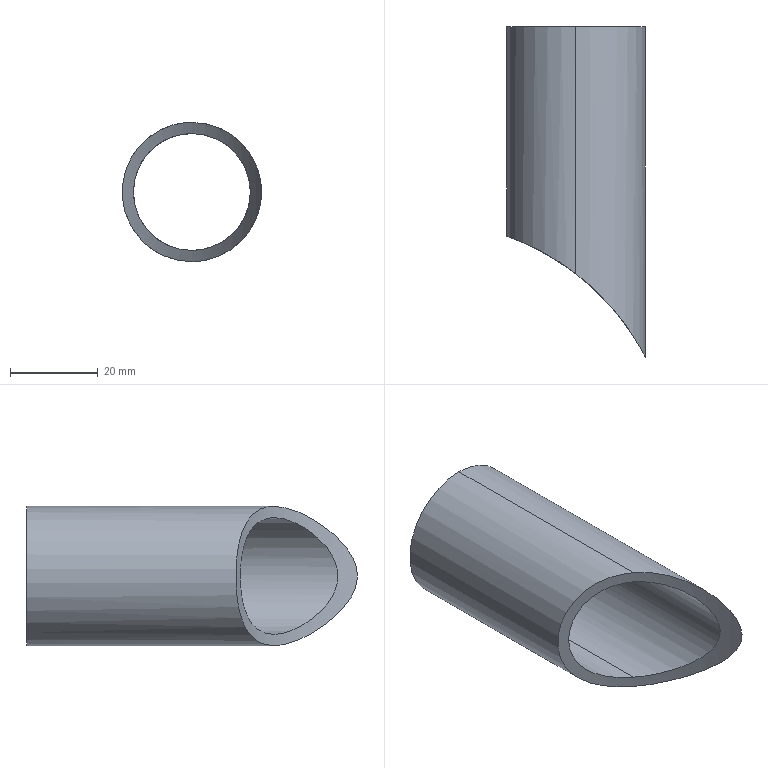Part | SolidWorks | features Extrusion 1 | 1 solid | 6 faces | box 31.75 x 75.418 x 31.75 mm | volume 13690 mm3 | cylinder 5 | plane 1 | commonest cylinder face diameters 26.645 x2 31.75 x2 114.3 x1
STEP:
#1=CARTESIAN_POINT('',(34.925,45.237,-203.822));
#2=VERTEX_POINT('',#1);
#3=CARTESIAN_POINT('',(34.925,45.237,-177.178));
#4=VERTEX_POINT('',#3);
#5=CARTESIAN_POINT('',(34.925,45.237,-203.822));
#6=CARTESIAN_POINT('',(34.177,45.814,-203.822));
#7=CARTESIAN_POINT('',(33.42,46.369,-203.76));
#8=CARTESIAN_POINT('',(32.272,47.169,-203.561));
#9=CARTESIAN_POINT('',(31.887,47.429,-203.477));
#10=CARTESIAN_POINT('',(31.114,47.94,-203.272));
#11=CARTESIAN_POINT('',(30.725,48.19,-203.15));
#12=CARTESIAN_POINT('',(29.574,48.911,-202.728));
#13=CARTESIAN_POINT('',(28.824,49.356,-202.373));
#14=CARTESIAN_POINT('',(27.729,49.974,-201.72));
#15=CARTESIAN_POINT('',(27.37,50.171,-201.482));
#16=CARTESIAN_POINT('',(26.664,50.55,-200.961));
#17=CARTESIAN_POINT('',(26.324,50.728,-200.683));
#18=CARTESIAN_POINT('',(25.343,51.229,-199.797));
#19=CARTESIAN_POINT('',(24.741,51.52,-199.138));
#20=CARTESIAN_POINT('',(23.93,51.9,-198.036));
#21=CARTESIAN_POINT('',(23.673,52.017,-197.648));
#22=CARTESIAN_POINT('',(23.204,52.228,-196.849));
#23=CARTESIAN_POINT('',(22.99,52.322,-196.438));
#24=CARTESIAN_POINT('',(22.607,52.489,-195.595));
#25=CARTESIAN_POINT('',(22.436,52.562,-195.162));
#26=CARTESIAN_POINT('',(22.14,52.688,-194.273));
#27=CARTESIAN_POINT('',(22.013,52.741,-193.815));
#28=CARTESIAN_POINT('',(21.708,52.867,-192.423));
#29=CARTESIAN_POINT('',(21.606,52.909,-191.486));
#30=CARTESIAN_POINT('',(21.601,52.91,-190.067));
#31=CARTESIAN_POINT('',(21.625,52.901,-189.589));
#32=CARTESIAN_POINT('',(21.724,52.86,-188.641));
#33=CARTESIAN_POINT('',(21.799,52.829,-188.174));
#34=CARTESIAN_POINT('',(21.996,52.748,-187.255));
#35=CARTESIAN_POINT('',(22.118,52.697,-186.801));
#36=CARTESIAN_POINT('',(22.41,52.573,-185.909));
#37=CARTESIAN_POINT('',(22.581,52.5,-185.467));
#38=CARTESIAN_POINT('',(23.158,52.25,-184.184));
#39=CARTESIAN_POINT('',(23.622,52.043,-183.389));
#40=CARTESIAN_POINT('',(24.43,51.666,-182.281));
#41=CARTESIAN_POINT('',(24.72,51.528,-181.924));
#42=CARTESIAN_POINT('',(25.325,51.233,-181.252));
#43=CARTESIAN_POINT('',(25.641,51.076,-180.935));
#44=CARTESIAN_POINT('',(26.295,50.743,-180.341));
#45=CARTESIAN_POINT('',(26.634,50.566,-180.063));
#46=CARTESIAN_POINT('',(27.333,50.192,-179.544));
#47=CARTESIAN_POINT('',(27.695,49.993,-179.302));
#48=CARTESIAN_POINT('',(28.797,49.372,-178.64));
#49=CARTESIAN_POINT('',(29.55,48.926,-178.283));
#50=CARTESIAN_POINT('',(31.082,47.967,-177.718));
#51=CARTESIAN_POINT('',(31.865,47.451,-177.51));
#52=CARTESIAN_POINT('',(33.406,46.379,-177.241));
#53=CARTESIAN_POINT('',(34.17,45.82,-177.178));
#54=CARTESIAN_POINT('',(34.925,45.237,-177.178));
#55=B_SPLINE_CURVE_WITH_KNOTS('',3,(#5,#6,#7,#8,#9,#10,#11,#12,#13,#14,#15,#16,#17,#18,#19,#20,#21,#22,#23,#24,#25,#26,#27,#28,#29,#30,#31,#32,#33,#34,#35,#36,#37,#38,#39,#40,#41,#42,#43,#44,#45,#46,#47,#48,#49,#50,#51,#52,#53,#54),.UNSPECIFIED.,.F.,.F.,(4,2,2,2,2,2,2,2,2,2,2,2,2,2,2,2,2,2,2,2,2,2,2,2,4),(0.0517,0.05452,0.05593,0.05735,0.06017,0.06159,0.063,0.06582,0.06724,0.06865,0.07006,0.07148,0.0743,0.07571,0.07713,0.07854,0.07995,0.08278,0.08419,0.0856,0.08702,0.08843,0.09126,0.09408,0.09691),.UNSPECIFIED.);
#56=EDGE_CURVE('',#2,#4,#55,.T.);
#57=ORIENTED_EDGE('',*,*,#56,.F.);
#58=CARTESIAN_POINT('',(34.925,101.6,-203.822));
#59=VERTEX_POINT('',#58);
#60=CARTESIAN_POINT('',(34.925,-57.151,-203.822));
#61=DIRECTION('',(0.,1.,0.));
#62=VECTOR('',#61,1000.);
#63=LINE('',#60,#62);
#64=EDGE_CURVE('',#2,#59,#63,.T.);
#65=ORIENTED_EDGE('',*,*,#64,.T.);
#66=CARTESIAN_POINT('',(34.925,101.6,-177.178));
#67=VERTEX_POINT('',#66);
#68=CARTESIAN_POINT('',(34.925,101.6,-190.5));
#69=DIRECTION('',(0.,1.,0.));
#70=DIRECTION('',(0.,0.,1.));
#71=AXIS2_PLACEMENT_3D('',#68,#69,#70);
#72=CIRCLE('',#71,13.322);
#73=EDGE_CURVE('',#59,#67,#72,.T.);
#74=ORIENTED_EDGE('',*,*,#73,.T.);
#75=CARTESIAN_POINT('',(34.925,-57.151,-177.178));
#76=DIRECTION('',(0.,1.,0.));
#77=VECTOR('',#76,1000.);
#78=LINE('',#75,#77);
#79=EDGE_CURVE('',#4,#67,#78,.T.);
#80=ORIENTED_EDGE('',*,*,#79,.F.);
#81=EDGE_LOOP('',(#57,#65,#74,#80));
#82=FACE_OUTER_BOUND('',#81,.T.);
#83=CARTESIAN_POINT('',(34.925,-57.151,-190.5));
#84=DIRECTION('',(0.,1.,0.));
#85=DIRECTION('',(0.,0.,1.));
#86=AXIS2_PLACEMENT_3D('',#83,#84,#85);
#87=CYLINDRICAL_SURFACE('',#86,13.322);
#88=ADVANCED_FACE('',(#82),#87,.F.);
#89=CARTESIAN_POINT('',(34.925,45.237,-174.625));
#90=VERTEX_POINT('',#89);
#91=CARTESIAN_POINT('',(34.925,45.237,-206.375));
#92=VERTEX_POINT('',#91);
#93=CARTESIAN_POINT('',(34.925,45.237,-174.625));
#94=CARTESIAN_POINT('',(35.986,44.418,-174.625));
#95=CARTESIAN_POINT('',(37.003,43.573,-174.73));
#96=CARTESIAN_POINT('',(38.96,41.833,-175.114));
#97=CARTESIAN_POINT('',(39.899,40.938,-175.393));
#98=CARTESIAN_POINT('',(41.702,39.099,-176.111));
#99=CARTESIAN_POINT('',(42.551,38.172,-176.545));
#100=CARTESIAN_POINT('',(44.148,36.312,-177.545));
#101=CARTESIAN_POINT('',(44.898,35.378,-178.112));
#102=CARTESIAN_POINT('',(45.955,33.98,-179.073));
#103=CARTESIAN_POINT('',(46.296,33.513,-179.412));
#104=CARTESIAN_POINT('',(46.948,32.594,-180.122));
#105=CARTESIAN_POINT('',(47.259,32.14,-180.494));
#106=CARTESIAN_POINT('',(47.854,31.247,-181.275));
#107=CARTESIAN_POINT('',(48.137,30.809,-181.685));
#108=CARTESIAN_POINT('',(48.675,29.953,-182.549));
#109=CARTESIAN_POINT('',(48.929,29.534,-183.004));
#110=CARTESIAN_POINT('',(49.404,28.734,-183.967));
#111=CARTESIAN_POINT('',(49.621,28.355,-184.471));
#112=CARTESIAN_POINT('',(49.916,27.831,-185.269));
#113=CARTESIAN_POINT('',(50.009,27.664,-185.542));
#114=CARTESIAN_POINT('',(50.182,27.348,-186.105));
#115=CARTESIAN_POINT('',(50.263,27.198,-186.396));
#116=CARTESIAN_POINT('',(50.483,26.789,-187.286));
#117=CARTESIAN_POINT('',(50.6,26.568,-187.902));
#118=CARTESIAN_POINT('',(50.72,26.337,-188.872));
#119=CARTESIAN_POINT('',(50.751,26.278,-189.204));
#120=CARTESIAN_POINT('',(50.791,26.2,-189.866));
#121=CARTESIAN_POINT('',(50.81,26.162,-190.528));
#122=CARTESIAN_POINT('',(50.788,26.204,-191.189));
#123=CARTESIAN_POINT('',(50.746,26.286,-191.851));
#124=CARTESIAN_POINT('',(50.714,26.348,-192.183));
#125=CARTESIAN_POINT('',(50.591,26.585,-193.151));
#126=CARTESIAN_POINT('',(50.472,26.811,-193.77));
#127=CARTESIAN_POINT('',(50.173,27.365,-194.959));
#128=CARTESIAN_POINT('',(49.998,27.686,-195.515));
#129=CARTESIAN_POINT('',(49.604,28.386,-196.572));
#130=CARTESIAN_POINT('',(49.385,28.765,-197.073));
#131=CARTESIAN_POINT('',(48.909,29.567,-198.032));
#132=CARTESIAN_POINT('',(48.654,29.986,-198.487));
#133=CARTESIAN_POINT('',(48.116,30.841,-199.346));
#134=CARTESIAN_POINT('',(47.833,31.279,-199.754));
#135=CARTESIAN_POINT('',(46.943,32.614,-200.919));
#136=CARTESIAN_POINT('',(46.294,33.531,-201.621));
#137=CARTESIAN_POINT('',(45.236,34.931,-202.58));
#138=CARTESIAN_POINT('',(44.87,35.4,-202.883));
#139=CARTESIAN_POINT('',(44.118,36.333,-203.451));
#140=CARTESIAN_POINT('',(43.73,36.799,-203.718));
#141=CARTESIAN_POINT('',(42.532,38.192,-204.466));
#142=CARTESIAN_POINT('',(41.686,39.115,-204.896));
#143=CARTESIAN_POINT('',(40.34,40.487,-205.431));
#144=CARTESIAN_POINT('',(39.877,40.943,-205.591));
#145=CARTESIAN_POINT('',(38.935,41.84,-205.868));
#146=CARTESIAN_POINT('',(38.455,42.281,-205.985));
#147=CARTESIAN_POINT('',(36.989,43.585,-206.272));
#148=CARTESIAN_POINT('',(35.976,44.425,-206.375));
#149=CARTESIAN_POINT('',(34.925,45.237,-206.375));
#150=B_SPLINE_CURVE_WITH_KNOTS('',3,(#93,#94,#95,#96,#97,#98,#99,#100,#101,#102,#103,#104,#105,#106,#107,#108,#109,#110,#111,#112,#113,#114,#115,#116,#117,#118,#119,#120,#121,#122,#123,#124,#125,#126,#127,#128,#129,#130,#131,#132,#133,#134,#135,#136,#137,#138,#139,#140,#141,#142,#143,#144,#145,#146,#147,#148,#149),.UNSPECIFIED.,.F.,.F.,(4,2,2,2,2,2,2,2,2,2,2,2,2,2,1,2,2,2,2,2,2,2,2,2,2,2,2,2,4),(0.,0.003969,0.007939,0.01191,0.01588,0.01786,0.01985,0.02183,0.02382,0.0258,0.02679,0.02779,0.02977,0.03076,0.03175,0.03275,0.03374,0.03572,0.03771,0.03969,0.04168,0.04366,0.04763,0.04962,0.0516,0.05557,0.05756,0.05954,0.06351),.UNSPECIFIED.);
#151=EDGE_CURVE('',#90,#92,#150,.T.);
#152=ORIENTED_EDGE('',*,*,#151,.T.);
#153=CARTESIAN_POINT('',(34.925,101.6,-206.375));
#154=VERTEX_POINT('',#153);
#155=CARTESIAN_POINT('',(34.925,-57.151,-206.375));
#156=DIRECTION('',(0.,1.,0.));
#157=VECTOR('',#156,1000.);
#158=LINE('',#155,#157);
#159=EDGE_CURVE('',#92,#154,#158,.T.);
#160=ORIENTED_EDGE('',*,*,#159,.T.);
#161=CARTESIAN_POINT('',(34.925,101.6,-174.625));
#162=VERTEX_POINT('',#161);
#163=CARTESIAN_POINT('',(34.925,101.6,-190.5));
#164=DIRECTION('',(0.,1.,0.));
#165=DIRECTION('',(0.,0.,1.));
#166=AXIS2_PLACEMENT_3D('',#163,#164,#165);
#167=CIRCLE('',#166,15.875);
#168=EDGE_CURVE('',#162,#154,#167,.T.);
#169=ORIENTED_EDGE('',*,*,#168,.F.);
#170=CARTESIAN_POINT('',(34.925,-57.151,-174.625));
#171=DIRECTION('',(0.,1.,0.));
#172=VECTOR('',#171,1000.);
#173=LINE('',#170,#172);
#174=EDGE_CURVE('',#90,#162,#173,.T.);
#175=ORIENTED_EDGE('',*,*,#174,.F.);
#176=EDGE_LOOP('',(#152,#160,#169,#175));
#177=FACE_OUTER_BOUND('',#176,.T.);
#178=CARTESIAN_POINT('',(34.925,-57.151,-190.5));
#179=DIRECTION('',(0.,1.,0.));
#180=DIRECTION('',(0.,0.,1.));
#181=AXIS2_PLACEMENT_3D('',#178,#179,#180);
#182=CYLINDRICAL_SURFACE('',#181,15.875);
#183=ADVANCED_FACE('',(#177),#182,.T.);
#184=ORIENTED_EDGE('',*,*,#159,.F.);
#185=CARTESIAN_POINT('',(34.925,45.237,-206.375));
#186=CARTESIAN_POINT('',(34.482,45.579,-206.375));
#187=CARTESIAN_POINT('',(34.03,45.917,-206.356));
#188=CARTESIAN_POINT('',(33.122,46.577,-206.279));
#189=CARTESIAN_POINT('',(32.666,46.897,-206.22));
#190=CARTESIAN_POINT('',(31.297,47.832,-205.983));
#191=CARTESIAN_POINT('',(30.38,48.418,-205.742));
#192=CARTESIAN_POINT('',(29.005,49.245,-205.238));
#193=CARTESIAN_POINT('',(28.544,49.514,-205.045));
#194=CARTESIAN_POINT('',(27.64,50.024,-204.614));
#195=CARTESIAN_POINT('',(27.197,50.266,-204.376));
#196=CARTESIAN_POINT('',(25.894,50.957,-203.595));
#197=CARTESIAN_POINT('',(25.063,51.369,-202.985));
#198=CARTESIAN_POINT('',(23.885,51.921,-201.92));
#199=CARTESIAN_POINT('',(23.502,52.095,-201.537));
#200=CARTESIAN_POINT('',(22.78,52.415,-200.737));
#201=CARTESIAN_POINT('',(22.439,52.562,-200.319));
#202=CARTESIAN_POINT('',(21.48,52.964,-199.01));
#203=CARTESIAN_POINT('',(20.923,53.184,-198.065));
#204=CARTESIAN_POINT('',(20.001,53.538,-196.027));
#205=CARTESIAN_POINT('',(19.652,53.665,-194.972));
#206=CARTESIAN_POINT('',(19.296,53.794,-193.338));
#207=CARTESIAN_POINT('',(19.205,53.826,-192.785));
#208=CARTESIAN_POINT('',(19.082,53.87,-191.66));
#209=CARTESIAN_POINT('',(19.051,53.881,-191.098));
#210=CARTESIAN_POINT('',(19.047,53.882,-189.419));
#211=CARTESIAN_POINT('',(19.162,53.842,-188.307));
#212=CARTESIAN_POINT('',(19.631,53.673,-186.098));
#213=CARTESIAN_POINT('',(19.978,53.547,-185.039));
#214=CARTESIAN_POINT('',(20.654,53.288,-183.525));
#215=CARTESIAN_POINT('',(20.905,53.19,-183.032));
#216=CARTESIAN_POINT('',(21.461,52.968,-182.071));
#217=CARTESIAN_POINT('',(21.761,52.846,-181.61));
#218=CARTESIAN_POINT('',(22.72,52.444,-180.291));
#219=CARTESIAN_POINT('',(23.437,52.13,-179.491));
#220=CARTESIAN_POINT('',(25.018,51.391,-178.05));
#221=CARTESIAN_POINT('',(25.857,50.976,-177.43));
#222=CARTESIAN_POINT('',(27.166,50.283,-176.641));
#223=CARTESIAN_POINT('',(27.612,50.04,-176.401));
#224=CARTESIAN_POINT('',(28.52,49.528,-175.966));
#225=CARTESIAN_POINT('',(28.979,49.261,-175.772));
#226=CARTESIAN_POINT('',(30.355,48.434,-175.266));
#227=CARTESIAN_POINT('',(31.275,47.846,-175.022));
#228=CARTESIAN_POINT('',(32.654,46.905,-174.781));
#229=CARTESIAN_POINT('',(33.115,46.581,-174.722));
#230=CARTESIAN_POINT('',(34.026,45.92,-174.644));
#231=CARTESIAN_POINT('',(34.478,45.582,-174.625));
#232=CARTESIAN_POINT('',(34.925,45.237,-174.625));
#233=B_SPLINE_CURVE_WITH_KNOTS('',3,(#185,#186,#187,#188,#189,#190,#191,#192,#193,#194,#195,#196,#197,#198,#199,#200,#201,#202,#203,#204,#205,#206,#207,#208,#209,#210,#211,#212,#213,#214,#215,#216,#217,#218,#219,#220,#221,#222,#223,#224,#225,#226,#227,#228,#229,#230,#231,#232),.UNSPECIFIED.,.F.,.F.,(4,2,2,2,2,2,2,2,2,2,2,2,2,2,2,2,2,2,2,2,2,2,2,4),(0.06351,0.06518,0.06685,0.0702,0.07187,0.07355,0.07689,0.07856,0.08024,0.08358,0.08693,0.0886,0.09027,0.09362,0.09696,0.09864,0.1003,0.1037,0.107,0.1087,0.1103,0.1137,0.1154,0.117),.UNSPECIFIED.);
#234=EDGE_CURVE('',#92,#90,#233,.T.);
#235=ORIENTED_EDGE('',*,*,#234,.T.);
#236=ORIENTED_EDGE('',*,*,#174,.T.);
#237=CARTESIAN_POINT('',(34.925,101.6,-190.5));
#238=DIRECTION('',(0.,1.,0.));
#239=DIRECTION('',(0.,0.,1.));
#240=AXIS2_PLACEMENT_3D('',#237,#238,#239);
#241=CIRCLE('',#240,15.875);
#242=EDGE_CURVE('',#154,#162,#241,.T.);
#243=ORIENTED_EDGE('',*,*,#242,.F.);
#244=EDGE_LOOP('',(#184,#235,#236,#243));
#245=FACE_OUTER_BOUND('',#244,.T.);
#246=CARTESIAN_POINT('',(34.925,-57.151,-190.5));
#247=DIRECTION('',(0.,1.,0.));
#248=DIRECTION('',(0.,0.,1.));
#249=AXIS2_PLACEMENT_3D('',#246,#247,#248);
#250=CYLINDRICAL_SURFACE('',#249,15.875);
#251=ADVANCED_FACE('',(#245),#250,.T.);
#252=CARTESIAN_POINT('',(34.925,101.6,-190.5));
#253=DIRECTION('',(0.,1.,0.));
#254=DIRECTION('',(0.,0.,1.));
#255=AXIS2_PLACEMENT_3D('',#252,#253,#254);
#256=CIRCLE('',#255,13.322);
#257=EDGE_CURVE('',#67,#59,#256,.T.);
#258=ORIENTED_EDGE('',*,*,#257,.F.);
#259=ORIENTED_EDGE('',*,*,#73,.F.);
#260=EDGE_LOOP('',(#258,#259));
#261=FACE_BOUND('',#260,.T.);
#262=ORIENTED_EDGE('',*,*,#168,.T.);
#263=ORIENTED_EDGE('',*,*,#242,.T.);
#264=EDGE_LOOP('',(#262,#263));
#265=FACE_OUTER_BOUND('',#264,.T.);
#266=CARTESIAN_POINT('',(34.925,101.6,-190.5));
#267=DIRECTION('',(0.,1.,0.));
#268=DIRECTION('',(0.,0.,1.));
#269=AXIS2_PLACEMENT_3D('',#266,#267,#268);
#270=PLANE('',#269);
#271=ADVANCED_FACE('',(#261,#265),#270,.T.);
#272=ORIENTED_EDGE('',*,*,#64,.F.);
#273=CARTESIAN_POINT('',(34.925,45.237,-177.178));
#274=CARTESIAN_POINT('',(35.788,44.57,-177.178));
#275=CARTESIAN_POINT('',(36.621,43.888,-177.261));
#276=CARTESIAN_POINT('',(38.232,42.492,-177.569));
#277=CARTESIAN_POINT('',(39.01,41.778,-177.794));
#278=CARTESIAN_POINT('',(40.138,40.685,-178.233));
#279=CARTESIAN_POINT('',(40.506,40.319,-178.397));
#280=CARTESIAN_POINT('',(41.22,39.589,-178.752));
#281=CARTESIAN_POINT('',(41.567,39.224,-178.945));
#282=CARTESIAN_POINT('',(42.581,38.131,-179.568));
#283=CARTESIAN_POINT('',(43.219,37.405,-180.043));
#284=CARTESIAN_POINT('',(44.121,36.327,-180.853));
#285=CARTESIAN_POINT('',(44.414,35.968,-181.14));
#286=CARTESIAN_POINT('',(44.977,35.262,-181.747));
#287=CARTESIAN_POINT('',(45.246,34.916,-182.065));
#288=CARTESIAN_POINT('',(45.759,34.241,-182.735));
#289=CARTESIAN_POINT('',(46.003,33.911,-183.087));
#290=CARTESIAN_POINT('',(46.466,33.275,-183.83));
#291=CARTESIAN_POINT('',(46.685,32.966,-184.223));
#292=CARTESIAN_POINT('',(47.091,32.384,-185.051));
#293=CARTESIAN_POINT('',(47.276,32.113,-185.482));
#294=CARTESIAN_POINT('',(47.606,31.621,-186.388));
#295=CARTESIAN_POINT('',(47.752,31.4,-186.864));
#296=CARTESIAN_POINT('',(47.994,31.028,-187.865));
#297=CARTESIAN_POINT('',(48.088,30.882,-188.378));
#298=CARTESIAN_POINT('',(48.184,30.732,-189.172));
#299=CARTESIAN_POINT('',(48.208,30.694,-189.44));
#300=CARTESIAN_POINT('',(48.24,30.643,-189.985));
#301=CARTESIAN_POINT('',(48.248,30.631,-190.259));
#302=CARTESIAN_POINT('',(48.246,30.634,-191.072));
#303=CARTESIAN_POINT('',(48.212,30.688,-191.608));
#304=CARTESIAN_POINT('',(48.113,30.843,-192.406));
#305=CARTESIAN_POINT('',(48.072,30.907,-192.671));
#306=CARTESIAN_POINT('',(47.976,31.055,-193.185));
#307=CARTESIAN_POINT('',(47.922,31.139,-193.437));
#308=CARTESIAN_POINT('',(47.74,31.418,-194.177));
#309=CARTESIAN_POINT('',(47.594,31.639,-194.649));
#310=CARTESIAN_POINT('',(47.258,32.139,-195.562));
#311=CARTESIAN_POINT('',(47.071,32.412,-195.992));
#312=CARTESIAN_POINT('',(46.667,32.991,-196.809));
#313=CARTESIAN_POINT('',(46.45,33.297,-197.197));
#314=CARTESIAN_POINT('',(45.987,33.933,-197.937));
#315=CARTESIAN_POINT('',(45.741,34.265,-198.29));
#316=CARTESIAN_POINT('',(44.964,35.286,-199.299));
#317=CARTESIAN_POINT('',(44.405,35.988,-199.894));
#318=CARTESIAN_POINT('',(43.209,37.416,-200.964));
#319=CARTESIAN_POINT('',(42.572,38.141,-201.438));
#320=CARTESIAN_POINT('',(41.553,39.239,-202.063));
#321=CARTESIAN_POINT('',(41.202,39.608,-202.258));
#322=CARTESIAN_POINT('',(40.487,40.338,-202.612));
#323=CARTESIAN_POINT('',(40.123,40.701,-202.773));
#324=CARTESIAN_POINT('',(39.007,41.781,-203.207));
#325=CARTESIAN_POINT('',(38.234,42.49,-203.431));
#326=CARTESIAN_POINT('',(37.027,43.536,-203.662));
#327=CARTESIAN_POINT('',(36.617,43.882,-203.721));
#328=CARTESIAN_POINT('',(35.779,44.568,-203.802));
#329=CARTESIAN_POINT('',(35.353,44.907,-203.822));
#330=CARTESIAN_POINT('',(34.925,45.237,-203.822));
#331=B_SPLINE_CURVE_WITH_KNOTS('',3,(#273,#274,#275,#276,#277,#278,#279,#280,#281,#282,#283,#284,#285,#286,#287,#288,#289,#290,#291,#292,#293,#294,#295,#296,#297,#298,#299,#300,#301,#302,#303,#304,#305,#306,#307,#308,#309,#310,#311,#312,#313,#314,#315,#316,#317,#318,#319,#320,#321,#322,#323,#324,#325,#326,#327,#328,#329,#330),.UNSPECIFIED.,.F.,.F.,(4,2,2,2,2,2,2,2,2,2,2,2,2,2,2,2,2,2,2,2,2,2,2,2,2,2,2,2,4),(0.,0.003231,0.006462,0.008078,0.009693,0.01292,0.01454,0.01616,0.01777,0.01939,0.021,0.02262,0.02423,0.02504,0.02585,0.02746,0.02827,0.02908,0.03069,0.03231,0.03393,0.03554,0.03877,0.042,0.04362,0.04523,0.04847,0.05008,0.0517),.UNSPECIFIED.);
#332=EDGE_CURVE('',#4,#2,#331,.T.);
#333=ORIENTED_EDGE('',*,*,#332,.F.);
#334=ORIENTED_EDGE('',*,*,#79,.T.);
#335=ORIENTED_EDGE('',*,*,#257,.T.);
#336=EDGE_LOOP('',(#272,#333,#334,#335));
#337=FACE_OUTER_BOUND('',#336,.T.);
#338=CARTESIAN_POINT('',(34.925,-57.151,-190.5));
#339=DIRECTION('',(0.,1.,0.));
#340=DIRECTION('',(0.,0.,1.));
#341=AXIS2_PLACEMENT_3D('',#338,#339,#340);
#342=CYLINDRICAL_SURFACE('',#341,13.322);
#343=ADVANCED_FACE('',(#337),#342,.F.);
#344=ORIENTED_EDGE('',*,*,#151,.F.);
#345=ORIENTED_EDGE('',*,*,#234,.F.);
#346=EDGE_LOOP('',(#344,#345));
#347=FACE_OUTER_BOUND('',#346,.T.);
#348=ORIENTED_EDGE('',*,*,#332,.T.);
#349=ORIENTED_EDGE('',*,*,#56,.T.);
#350=EDGE_LOOP('',(#348,#349));
#351=FACE_BOUND('',#350,.T.);
#352=CARTESIAN_POINT('',(0.,0.,222.25));
#353=DIRECTION('',(0.,0.,-1.));
#354=DIRECTION('',(-1.,0.,0.));
#355=AXIS2_PLACEMENT_3D('',#352,#353,#354);
#356=CYLINDRICAL_SURFACE('',#355,57.15);
#357=ADVANCED_FACE('',(#347,#351),#356,.F.);
#358=CLOSED_SHELL('',(#88,#183,#251,#271,#343,#357));
#359=MANIFOLD_SOLID_BREP('',#358);
#360=CARTESIAN_POINT('',(0.,0.,0.));
#361=DIRECTION('',(0.,0.,1.));
#362=DIRECTION('',(1.,0.,0.));
#363=AXIS2_PLACEMENT_3D('',#360,#361,#362);
#364=(LENGTH_UNIT()NAMED_UNIT(*)SI_UNIT(.MILLI.,.METRE.));
#365=UNCERTAINTY_MEASURE_WITH_UNIT(LENGTH_MEASURE(0.00001),#364,'','');
#366=(NAMED_UNIT(*)PLANE_ANGLE_UNIT()SI_UNIT($,.RADIAN.));
#367=(NAMED_UNIT(*)SI_UNIT($,.STERADIAN.)SOLID_ANGLE_UNIT());
#368=(GEOMETRIC_REPRESENTATION_CONTEXT(3)GLOBAL_UNCERTAINTY_ASSIGNED_CONTEXT((#365))GLOBAL_UNIT_ASSIGNED_CONTEXT((#364,#366,#367))REPRESENTATION_CONTEXT('',''));
#369=ADVANCED_BREP_SHAPE_REPRESENTATION('',(#359,#363),#368);